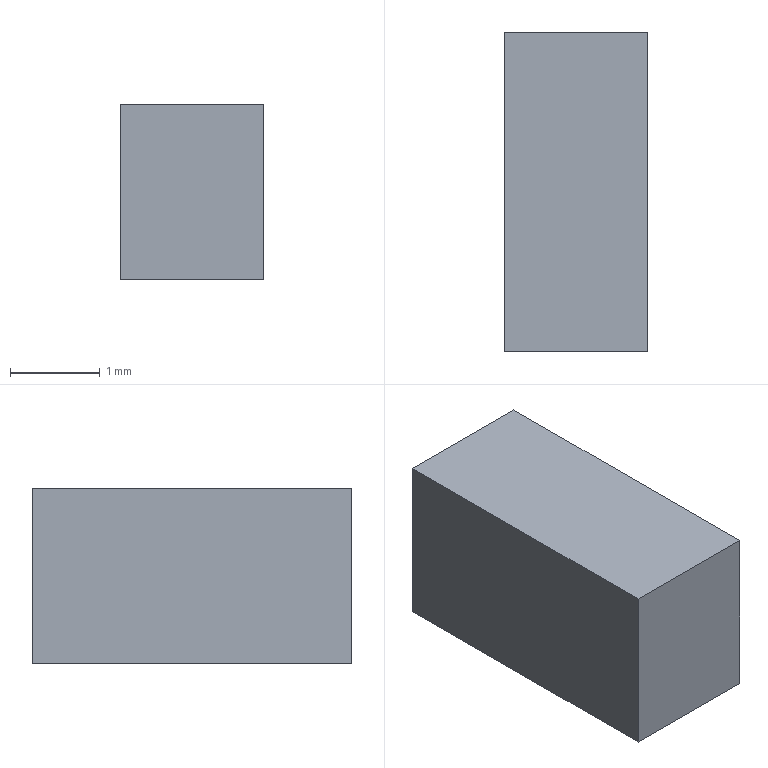Part | Creo | 1 solid | 6 faces | box 1.6 x 3.567 x 1.955 mm | volume 11.154 mm3 | plane 6
STEP:
#1=CARTESIAN_POINT('',(0.,0.,0.));
#2=DIRECTION('',(0.,0.,1.));
#3=DIRECTION('',(1.,0.,0.));
#4=AXIS2_PLACEMENT_3D('',#1,#2,#3);
#5=CARTESIAN_POINT('',(-0.8,-1.783,0.));
#6=VERTEX_POINT('',#5);
#7=CARTESIAN_POINT('',(0.8,-1.783,0.));
#8=VERTEX_POINT('',#7);
#9=CARTESIAN_POINT('',(-0.8,-1.783,0.));
#10=DIRECTION('',(1.,0.,0.));
#11=VECTOR('',#10,1.6);
#12=LINE('',#9,#11);
#13=EDGE_CURVE('',#6,#8,#12,.T.);
#14=ORIENTED_EDGE('',*,*,#13,.T.);
#15=CARTESIAN_POINT('',(0.8,1.783,0.));
#16=VERTEX_POINT('',#15);
#17=CARTESIAN_POINT('',(0.8,-1.783,0.));
#18=DIRECTION('',(0.,1.,0.));
#19=VECTOR('',#18,3.567);
#20=LINE('',#17,#19);
#21=EDGE_CURVE('',#8,#16,#20,.T.);
#22=ORIENTED_EDGE('',*,*,#21,.T.);
#23=CARTESIAN_POINT('',(-0.8,1.783,0.));
#24=VERTEX_POINT('',#23);
#25=CARTESIAN_POINT('',(0.8,1.783,0.));
#26=DIRECTION('',(-1.,0.,0.));
#27=VECTOR('',#26,1.6);
#28=LINE('',#25,#27);
#29=EDGE_CURVE('',#16,#24,#28,.T.);
#30=ORIENTED_EDGE('',*,*,#29,.T.);
#31=CARTESIAN_POINT('',(-0.8,1.783,0.));
#32=DIRECTION('',(0.,-1.,0.));
#33=VECTOR('',#32,3.567);
#34=LINE('',#31,#33);
#35=EDGE_CURVE('',#24,#6,#34,.T.);
#36=ORIENTED_EDGE('',*,*,#35,.T.);
#37=EDGE_LOOP('',(#14,#22,#30,#36));
#38=FACE_OUTER_BOUND('',#37,.F.);
#39=CARTESIAN_POINT('',(0.,0.,0.));
#40=DIRECTION('',(0.,0.,1.));
#41=DIRECTION('',(1.,0.,0.));
#42=AXIS2_PLACEMENT_3D('',#39,#40,#41);
#43=PLANE('',#42);
#44=ADVANCED_FACE('',(#38),#43,.F.);
#45=ORIENTED_EDGE('',*,*,#13,.F.);
#46=CARTESIAN_POINT('',(-0.8,-1.783,1.955));
#47=VERTEX_POINT('',#46);
#48=CARTESIAN_POINT('',(-0.8,-1.783,0.));
#49=DIRECTION('',(0.,0.,1.));
#50=VECTOR('',#49,1.955);
#51=LINE('',#48,#50);
#52=EDGE_CURVE('',#6,#47,#51,.T.);
#53=ORIENTED_EDGE('',*,*,#52,.T.);
#54=CARTESIAN_POINT('',(0.8,-1.783,1.955));
#55=VERTEX_POINT('',#54);
#56=CARTESIAN_POINT('',(-0.8,-1.783,1.955));
#57=DIRECTION('',(1.,0.,0.));
#58=VECTOR('',#57,1.6);
#59=LINE('',#56,#58);
#60=EDGE_CURVE('',#47,#55,#59,.T.);
#61=ORIENTED_EDGE('',*,*,#60,.T.);
#62=CARTESIAN_POINT('',(0.8,-1.783,0.));
#63=DIRECTION('',(0.,0.,1.));
#64=VECTOR('',#63,1.955);
#65=LINE('',#62,#64);
#66=EDGE_CURVE('',#8,#55,#65,.T.);
#67=ORIENTED_EDGE('',*,*,#66,.F.);
#68=EDGE_LOOP('',(#45,#53,#61,#67));
#69=FACE_OUTER_BOUND('',#68,.F.);
#70=CARTESIAN_POINT('',(-0.8,-1.783,0.));
#71=DIRECTION('',(0.,-1.,0.));
#72=DIRECTION('',(1.,0.,0.));
#73=AXIS2_PLACEMENT_3D('',#70,#71,#72);
#74=PLANE('',#73);
#75=ADVANCED_FACE('',(#69),#74,.T.);
#76=ORIENTED_EDGE('',*,*,#35,.F.);
#77=CARTESIAN_POINT('',(-0.8,1.783,1.955));
#78=VERTEX_POINT('',#77);
#79=CARTESIAN_POINT('',(-0.8,1.783,0.));
#80=DIRECTION('',(0.,0.,1.));
#81=VECTOR('',#80,1.955);
#82=LINE('',#79,#81);
#83=EDGE_CURVE('',#24,#78,#82,.T.);
#84=ORIENTED_EDGE('',*,*,#83,.T.);
#85=CARTESIAN_POINT('',(-0.8,1.783,1.955));
#86=DIRECTION('',(0.,-1.,0.));
#87=VECTOR('',#86,3.567);
#88=LINE('',#85,#87);
#89=EDGE_CURVE('',#78,#47,#88,.T.);
#90=ORIENTED_EDGE('',*,*,#89,.T.);
#91=ORIENTED_EDGE('',*,*,#52,.F.);
#92=EDGE_LOOP('',(#76,#84,#90,#91));
#93=FACE_OUTER_BOUND('',#92,.F.);
#94=CARTESIAN_POINT('',(-0.8,1.783,0.));
#95=DIRECTION('',(-1.,0.,0.));
#96=DIRECTION('',(0.,-1.,0.));
#97=AXIS2_PLACEMENT_3D('',#94,#95,#96);
#98=PLANE('',#97);
#99=ADVANCED_FACE('',(#93),#98,.T.);
#100=ORIENTED_EDGE('',*,*,#29,.F.);
#101=CARTESIAN_POINT('',(0.8,1.783,1.955));
#102=VERTEX_POINT('',#101);
#103=CARTESIAN_POINT('',(0.8,1.783,0.));
#104=DIRECTION('',(0.,0.,1.));
#105=VECTOR('',#104,1.955);
#106=LINE('',#103,#105);
#107=EDGE_CURVE('',#16,#102,#106,.T.);
#108=ORIENTED_EDGE('',*,*,#107,.T.);
#109=CARTESIAN_POINT('',(0.8,1.783,1.955));
#110=DIRECTION('',(-1.,0.,0.));
#111=VECTOR('',#110,1.6);
#112=LINE('',#109,#111);
#113=EDGE_CURVE('',#102,#78,#112,.T.);
#114=ORIENTED_EDGE('',*,*,#113,.T.);
#115=ORIENTED_EDGE('',*,*,#83,.F.);
#116=EDGE_LOOP('',(#100,#108,#114,#115));
#117=FACE_OUTER_BOUND('',#116,.F.);
#118=CARTESIAN_POINT('',(0.8,1.783,0.));
#119=DIRECTION('',(0.,1.,0.));
#120=DIRECTION('',(-1.,0.,0.));
#121=AXIS2_PLACEMENT_3D('',#118,#119,#120);
#122=PLANE('',#121);
#123=ADVANCED_FACE('',(#117),#122,.T.);
#124=ORIENTED_EDGE('',*,*,#21,.F.);
#125=ORIENTED_EDGE('',*,*,#66,.T.);
#126=CARTESIAN_POINT('',(0.8,-1.783,1.955));
#127=DIRECTION('',(0.,1.,0.));
#128=VECTOR('',#127,3.567);
#129=LINE('',#126,#128);
#130=EDGE_CURVE('',#55,#102,#129,.T.);
#131=ORIENTED_EDGE('',*,*,#130,.T.);
#132=ORIENTED_EDGE('',*,*,#107,.F.);
#133=EDGE_LOOP('',(#124,#125,#131,#132));
#134=FACE_OUTER_BOUND('',#133,.F.);
#135=CARTESIAN_POINT('',(0.8,-1.783,0.));
#136=DIRECTION('',(1.,0.,0.));
#137=DIRECTION('',(0.,1.,0.));
#138=AXIS2_PLACEMENT_3D('',#135,#136,#137);
#139=PLANE('',#138);
#140=ADVANCED_FACE('',(#134),#139,.T.);
#141=ORIENTED_EDGE('',*,*,#60,.F.);
#142=ORIENTED_EDGE('',*,*,#89,.F.);
#143=ORIENTED_EDGE('',*,*,#113,.F.);
#144=ORIENTED_EDGE('',*,*,#130,.F.);
#145=EDGE_LOOP('',(#141,#142,#143,#144));
#146=FACE_OUTER_BOUND('',#145,.F.);
#147=CARTESIAN_POINT('',(0.,0.,1.955));
#148=DIRECTION('',(0.,0.,1.));
#149=DIRECTION('',(1.,0.,0.));
#150=AXIS2_PLACEMENT_3D('',#147,#148,#149);
#151=PLANE('',#150);
#152=ADVANCED_FACE('',(#146),#151,.T.);
#153=CLOSED_SHELL('',(#44,#75,#99,#123,#140,#152));
#154=MANIFOLD_SOLID_BREP('',#153);
#155=(LENGTH_UNIT()NAMED_UNIT(*)SI_UNIT(.MILLI.,.METRE.));
#156=UNCERTAINTY_MEASURE_WITH_UNIT(LENGTH_MEASURE(0.000437),#155,'','');
#157=(NAMED_UNIT(*)PLANE_ANGLE_UNIT()SI_UNIT($,.RADIAN.));
#158=PLANE_ANGLE_MEASURE_WITH_UNIT(PLANE_ANGLE_MEASURE(0.01745),#157);
#159=(CONVERSION_BASED_UNIT('DEGREE',#158)NAMED_UNIT(*)PLANE_ANGLE_UNIT());
#160=(NAMED_UNIT(*)SI_UNIT($,.STERADIAN.)SOLID_ANGLE_UNIT());
#161=(GEOMETRIC_REPRESENTATION_CONTEXT(3)GLOBAL_UNCERTAINTY_ASSIGNED_CONTEXT((#156))GLOBAL_UNIT_ASSIGNED_CONTEXT((#155,#159,#160))REPRESENTATION_CONTEXT('',''));
#162=ADVANCED_BREP_SHAPE_REPRESENTATION('',(#4,#154),#161);